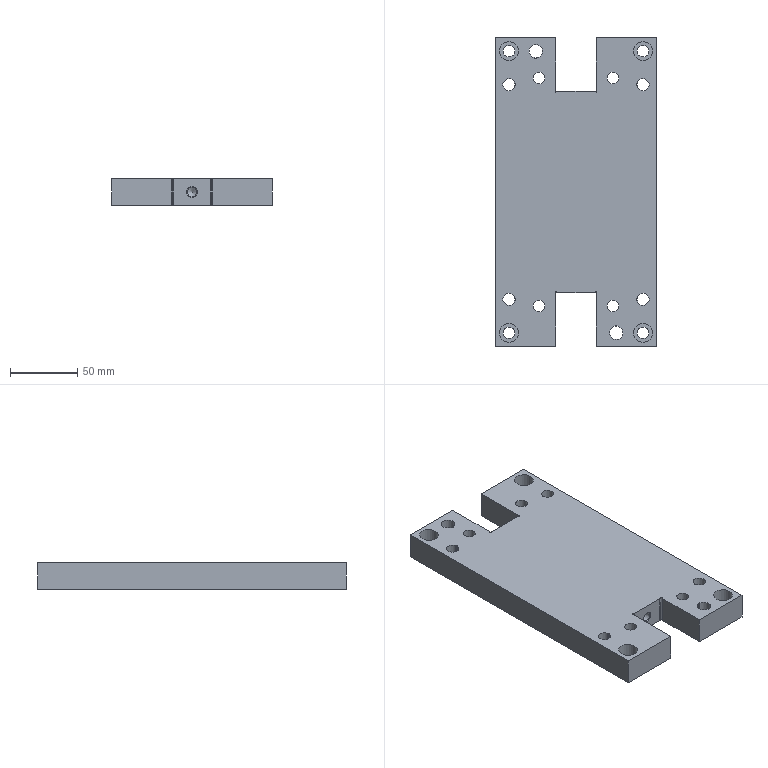Part | STEP file | YBQDJ-YY-1 | 1 solid | 82 faces | box 120 x 230 x 20 mm | volume 476492 mm3 | cylinder 52 | plane 22 | cone 8 | commonest cylinder face diameters 4 x18 1 x10 8.7 x8 14 x8 9 x4 6.8 x2